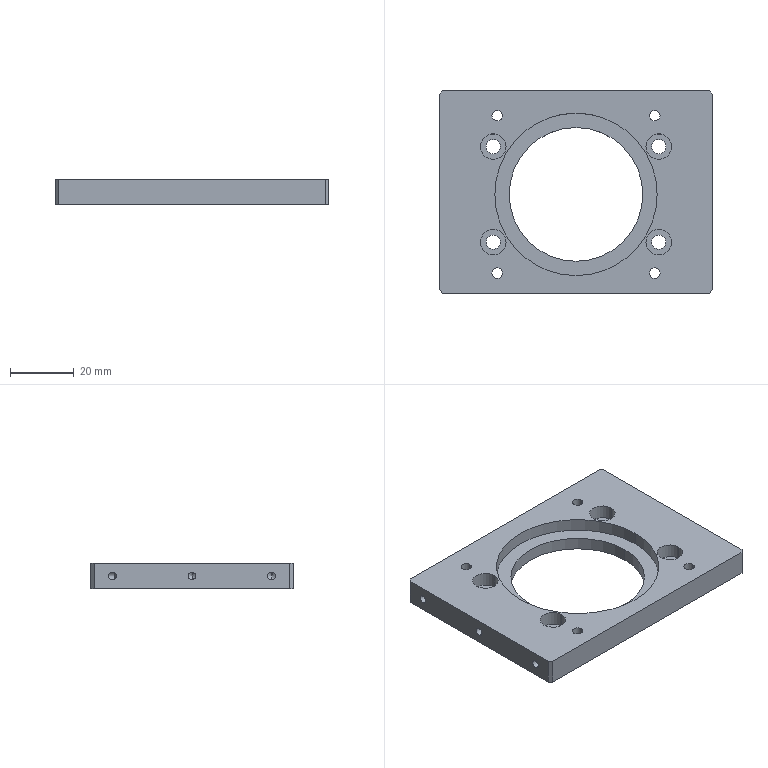Part | STEP file | 1 solid | 79 faces | box 86 x 63.5 x 8 mm | volume 28261 mm3 | cylinder 44 | cone 20 | plane 15 | commonest cylinder face diameters 2.5 x16 3.3 x8 4.5 x8 8 x8 42 x2 51 x2